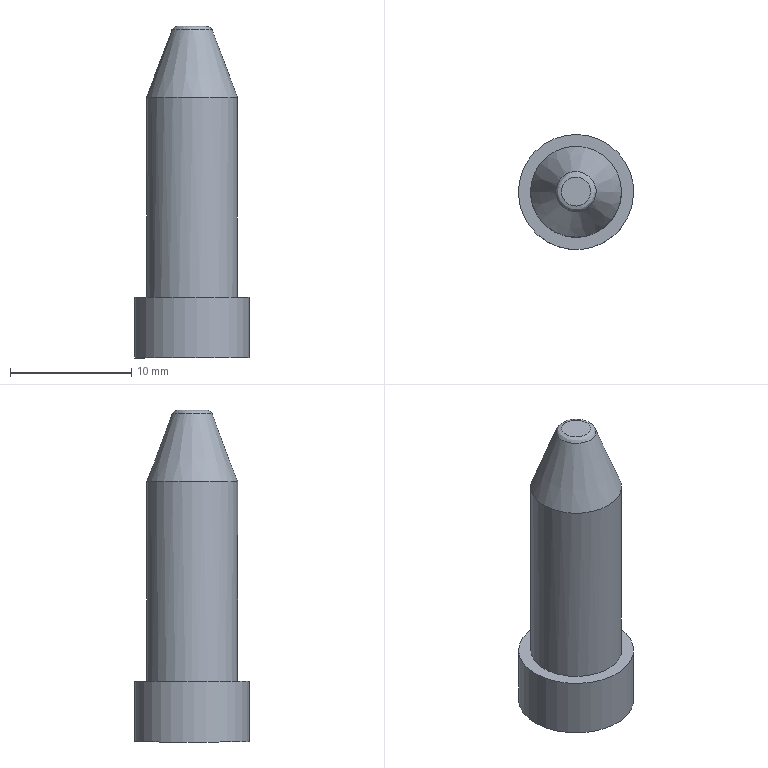Part | STEP file | gslz 2016.10.28-6_id1054_x_t | 1 solid | 7 faces | box 9.497 x 9.497 x 27.383 mm | volume 1219 mm3 | plane 3 | spline 2 | cylinder 1 | cone 1 | commonest cylinder face diameters 7.5 x1
STEP:
#1=CARTESIAN_POINT('',(19.769,170.458,47.));
#2=VERTEX_POINT('',#1);
#3=CARTESIAN_POINT('',(23.484,170.969,47.));
#4=DIRECTION('',(0.,0.,1.));
#5=DIRECTION('',(-0.9907,-0.1362,0.));
#6=AXIS2_PLACEMENT_3D('',#3,#4,#5);
#7=ELLIPSE('',#6,3.75,3.75);
#8=EDGE_CURVE('',#2,#2,#7,.T.);
#9=ORIENTED_EDGE('',*,*,#8,.T.);
#10=EDGE_LOOP('',(#9));
#11=FACE_BOUND('',#10,.T.);
#12=CARTESIAN_POINT('',(27.232,170.968,63.49));
#13=VERTEX_POINT('',#12);
#14=CARTESIAN_POINT('',(27.232,169.977,63.49));
#15=CARTESIAN_POINT('',(27.232,171.959,63.49));
#16=CARTESIAN_POINT('',(26.829,172.923,63.49));
#17=CARTESIAN_POINT('',(25.441,174.313,63.49));
#18=CARTESIAN_POINT('',(24.463,174.717,63.49));
#19=CARTESIAN_POINT('',(22.508,174.719,63.49));
#20=CARTESIAN_POINT('',(21.53,174.318,63.49));
#21=CARTESIAN_POINT('',(20.137,172.928,63.49));
#22=CARTESIAN_POINT('',(19.732,171.954,63.49));
#23=CARTESIAN_POINT('',(19.731,169.989,63.49));
#24=CARTESIAN_POINT('',(20.137,169.011,63.49));
#25=CARTESIAN_POINT('',(21.517,167.628,63.49));
#26=CARTESIAN_POINT('',(22.493,167.22,63.49));
#27=CARTESIAN_POINT('',(24.46,167.217,63.49));
#28=CARTESIAN_POINT('',(25.435,167.62,63.49));
#29=CARTESIAN_POINT('',(26.827,169.009,63.49));
#30=CARTESIAN_POINT('',(27.232,169.977,63.49));
#31=CARTESIAN_POINT('',(27.232,171.959,63.49));
#32=B_SPLINE_CURVE_WITH_KNOTS('',3,(#14,#15,#16,#17,#18,#19,#20,#21,#22,#23,#24,#25,#26,#27,#28,#29,#30,#31),.UNSPECIFIED.,.T.,.F.,(2,2,2,2,2,2,2,2,2,2,2),(-0.125,0.,0.125,0.25,0.375,0.5,0.625,0.75,0.875,1.,1.125),.UNSPECIFIED.);
#33=EDGE_CURVE('',#13,#13,#32,.T.);
#34=ORIENTED_EDGE('',*,*,#33,.F.);
#35=EDGE_LOOP('',(#34));
#36=FACE_BOUND('',#35,.T.);
#37=CARTESIAN_POINT('',(23.49,170.969,13.491));
#38=DIRECTION('',(-0.0001633,-0.00002245,1.));
#39=DIRECTION('',(1.,0.,0.0001633));
#40=AXIS2_PLACEMENT_3D('',#37,#38,#39);
#41=CYLINDRICAL_SURFACE('',#40,3.75);
#42=ADVANCED_FACE('',(#11,#36),#41,.T.);
#43=CARTESIAN_POINT('',(24.674,170.968,69.383));
#44=VERTEX_POINT('',#43);
#45=CARTESIAN_POINT('',(23.481,170.968,69.383));
#46=DIRECTION('',(0.0001633,-0.00002245,1.));
#47=DIRECTION('',(1.,-0.000000146,-0.0001633));
#48=AXIS2_PLACEMENT_3D('',#45,#46,#47);
#49=ELLIPSE('',#48,1.194,1.194);
#50=EDGE_CURVE('',#44,#44,#49,.T.);
#51=ORIENTED_EDGE('',*,*,#50,.T.);
#52=EDGE_LOOP('',(#51));
#53=FACE_OUTER_BOUND('',#52,.T.);
#54=CARTESIAN_POINT('',(-22.081,170.968,69.391));
#55=DIRECTION('',(0.0001633,-0.00002245,1.));
#56=DIRECTION('',(-1.,0.,0.0001633));
#57=AXIS2_PLACEMENT_3D('',#54,#55,#56);
#58=PLANE('',#57);
#59=ADVANCED_FACE('',(#53),#58,.T.);
#60=CARTESIAN_POINT('',(21.828,170.793,69.059));
#61=VERTEX_POINT('',#60);
#62=CARTESIAN_POINT('',(21.919,169.928,69.059));
#63=CARTESIAN_POINT('',(21.737,171.659,69.059));
#64=CARTESIAN_POINT('',(22.441,172.529,69.059));
#65=CARTESIAN_POINT('',(24.171,172.712,69.059));
#66=CARTESIAN_POINT('',(25.041,172.008,69.059));
#67=CARTESIAN_POINT('',(25.224,170.277,69.059));
#68=CARTESIAN_POINT('',(24.52,169.407,69.059));
#69=CARTESIAN_POINT('',(22.79,169.224,69.059));
#70=CARTESIAN_POINT('',(21.919,169.928,69.059));
#71=CARTESIAN_POINT('',(21.737,171.659,69.059));
#72=B_SPLINE_CURVE_WITH_KNOTS('',3,(#62,#63,#64,#65,#66,#67,#68,#69,#70,#71),.UNSPECIFIED.,.T.,.F.,(2,2,2,2,2,2,2),(-0.25,0.,0.25,0.5,0.75,1.,1.25),.UNSPECIFIED.);
#73=EDGE_CURVE('',#61,#61,#72,.T.);
#74=ORIENTED_EDGE('',*,*,#73,.T.);
#75=EDGE_LOOP('',(#74));
#76=FACE_BOUND('',#75,.T.);
#77=ORIENTED_EDGE('',*,*,#33,.T.);
#78=EDGE_LOOP('',(#77));
#79=FACE_BOUND('',#78,.T.);
#80=CARTESIAN_POINT('',(23.481,170.968,67.49));
#81=DIRECTION('',(0.0001633,0.00002245,-1.));
#82=DIRECTION('',(1.,-0.0000003,0.0001633));
#83=AXIS2_PLACEMENT_3D('',#80,#81,#82);
#84=CONICAL_SURFACE('',#83,2.25,20.556);
#85=ADVANCED_FACE('',(#76,#79),#84,.T.);
#86=CARTESIAN_POINT('',(18.873,169.831,47.));
#87=VERTEX_POINT('',#86);
#88=CARTESIAN_POINT('',(19.135,168.787,47.));
#89=CARTESIAN_POINT('',(18.833,169.993,47.));
#90=CARTESIAN_POINT('',(18.801,170.156,47.));
#91=CARTESIAN_POINT('',(18.609,171.554,47.));
#92=CARTESIAN_POINT('',(18.948,172.848,47.));
#93=CARTESIAN_POINT('',(20.451,174.829,47.));
#94=CARTESIAN_POINT('',(21.605,175.505,47.));
#95=CARTESIAN_POINT('',(24.069,175.844,47.));
#96=CARTESIAN_POINT('',(25.363,175.505,47.));
#97=CARTESIAN_POINT('',(27.345,174.002,47.));
#98=CARTESIAN_POINT('',(28.021,172.847,47.));
#99=CARTESIAN_POINT('',(28.359,170.383,47.));
#100=CARTESIAN_POINT('',(28.02,169.089,47.));
#101=CARTESIAN_POINT('',(26.518,167.108,47.));
#102=CARTESIAN_POINT('',(25.363,166.432,47.));
#103=CARTESIAN_POINT('',(22.899,166.093,47.));
#104=CARTESIAN_POINT('',(21.605,166.432,47.));
#105=CARTESIAN_POINT('',(19.756,167.834,47.));
#106=CARTESIAN_POINT('',(19.135,168.787,47.));
#107=CARTESIAN_POINT('',(18.833,169.993,47.));
#108=B_SPLINE_CURVE_WITH_KNOTS('',3,(#88,#89,#90,#91,#92,#93,#94,#95,#96,#97,#98,#99,#100,#101,#102,#103,#104,#105,#106,#107),.UNSPECIFIED.,.T.,.F.,(2,2,2,2,2,2,2,2,2,2,2,2),(-0.1082,0.,0.01676,0.1418,0.2668,0.3918,0.5168,0.6418,0.7668,0.8918,1.,1.017),.UNSPECIFIED.);
#109=EDGE_CURVE('',#87,#87,#108,.T.);
#110=ORIENTED_EDGE('',*,*,#109,.T.);
#111=EDGE_LOOP('',(#110));
#112=FACE_BOUND('',#111,.T.);
#113=CARTESIAN_POINT('',(18.873,169.831,42.));
#114=VERTEX_POINT('',#113);
#115=CARTESIAN_POINT('',(19.135,168.787,42.));
#116=CARTESIAN_POINT('',(18.833,169.993,42.));
#117=CARTESIAN_POINT('',(18.801,170.156,42.));
#118=CARTESIAN_POINT('',(18.609,171.554,42.));
#119=CARTESIAN_POINT('',(18.948,172.848,42.));
#120=CARTESIAN_POINT('',(20.451,174.829,42.));
#121=CARTESIAN_POINT('',(21.605,175.505,42.));
#122=CARTESIAN_POINT('',(24.069,175.844,42.));
#123=CARTESIAN_POINT('',(25.363,175.505,42.));
#124=CARTESIAN_POINT('',(27.345,174.002,42.));
#125=CARTESIAN_POINT('',(28.021,172.847,42.));
#126=CARTESIAN_POINT('',(28.359,170.383,42.));
#127=CARTESIAN_POINT('',(28.02,169.089,42.));
#128=CARTESIAN_POINT('',(26.518,167.108,42.));
#129=CARTESIAN_POINT('',(25.363,166.432,42.));
#130=CARTESIAN_POINT('',(22.899,166.093,42.));
#131=CARTESIAN_POINT('',(21.605,166.432,42.));
#132=CARTESIAN_POINT('',(19.756,167.834,42.));
#133=CARTESIAN_POINT('',(19.135,168.787,42.));
#134=CARTESIAN_POINT('',(18.833,169.993,42.));
#135=B_SPLINE_CURVE_WITH_KNOTS('',3,(#115,#116,#117,#118,#119,#120,#121,#122,#123,#124,#125,#126,#127,#128,#129,#130,#131,#132,#133,#134),.UNSPECIFIED.,.T.,.F.,(2,2,2,2,2,2,2,2,2,2,2,2),(-0.1082,0.,0.01676,0.1418,0.2668,0.3918,0.5168,0.6418,0.7668,0.8918,1.,1.017),.UNSPECIFIED.);
#136=EDGE_CURVE('',#114,#114,#135,.T.);
#137=ORIENTED_EDGE('',*,*,#136,.F.);
#138=EDGE_LOOP('',(#137));
#139=FACE_BOUND('',#138,.T.);
#140=CARTESIAN_POINT('',(18.948,169.09,47.));
#141=CARTESIAN_POINT('',(18.948,169.09,42.));
#142=CARTESIAN_POINT('',(18.609,171.554,47.));
#143=CARTESIAN_POINT('',(18.609,171.554,42.));
#144=CARTESIAN_POINT('',(18.948,172.848,47.));
#145=CARTESIAN_POINT('',(18.948,172.848,42.));
#146=CARTESIAN_POINT('',(20.451,174.829,47.));
#147=CARTESIAN_POINT('',(20.451,174.829,42.));
#148=CARTESIAN_POINT('',(21.605,175.505,47.));
#149=CARTESIAN_POINT('',(21.605,175.505,42.));
#150=CARTESIAN_POINT('',(24.069,175.844,47.));
#151=CARTESIAN_POINT('',(24.069,175.844,42.));
#152=CARTESIAN_POINT('',(25.363,175.505,47.));
#153=CARTESIAN_POINT('',(25.363,175.505,42.));
#154=CARTESIAN_POINT('',(27.345,174.002,47.));
#155=CARTESIAN_POINT('',(27.345,174.002,42.));
#156=CARTESIAN_POINT('',(28.021,172.847,47.));
#157=CARTESIAN_POINT('',(28.021,172.847,42.));
#158=CARTESIAN_POINT('',(28.359,170.383,47.));
#159=CARTESIAN_POINT('',(28.359,170.383,42.));
#160=CARTESIAN_POINT('',(28.02,169.089,47.));
#161=CARTESIAN_POINT('',(28.02,169.089,42.));
#162=CARTESIAN_POINT('',(26.518,167.108,47.));
#163=CARTESIAN_POINT('',(26.518,167.108,42.));
#164=CARTESIAN_POINT('',(25.363,166.432,47.));
#165=CARTESIAN_POINT('',(25.363,166.432,42.));
#166=CARTESIAN_POINT('',(22.899,166.093,47.));
#167=CARTESIAN_POINT('',(22.899,166.093,42.));
#168=CARTESIAN_POINT('',(21.605,166.432,47.));
#169=CARTESIAN_POINT('',(21.605,166.432,42.));
#170=CARTESIAN_POINT('',(19.623,167.935,47.));
#171=CARTESIAN_POINT('',(19.623,167.935,42.));
#172=CARTESIAN_POINT('',(18.948,169.09,47.));
#173=CARTESIAN_POINT('',(18.948,169.09,42.));
#174=CARTESIAN_POINT('',(18.609,171.554,47.));
#175=CARTESIAN_POINT('',(18.609,171.554,42.));
#176=B_SPLINE_SURFACE_WITH_KNOTS('',3,1,((#140,#141),(#142,#143),(#144,#145),(#146,#147),(#148,#149),(#150,#151),(#152,#153),(#154,#155),(#156,#157),(#158,#159),(#160,#161),(#162,#163),(#164,#165),(#166,#167),(#168,#169),(#170,#171),(#172,#173),(#174,#175)),.UNSPECIFIED.,.T.,.F.,.F.,(2,2,2,2,2,2,2,2,2,2,2),(2,2),(-0.125,0.,0.125,0.25,0.375,0.5,0.625,0.75,0.875,1.,1.125),(0.,1.),.UNSPECIFIED.);
#177=ADVANCED_FACE('',(#112,#139),#176,.T.);
#178=ORIENTED_EDGE('',*,*,#8,.F.);
#179=EDGE_LOOP('',(#178));
#180=FACE_BOUND('',#179,.T.);
#181=ORIENTED_EDGE('',*,*,#109,.F.);
#182=EDGE_LOOP('',(#181));
#183=FACE_BOUND('',#182,.T.);
#184=CARTESIAN_POINT('',(23.484,170.969,47.));
#185=DIRECTION('',(0.,0.,1.));
#186=DIRECTION('',(1.,-0.0000003,0.));
#187=AXIS2_PLACEMENT_3D('',#184,#185,#186);
#188=PLANE('',#187);
#189=ADVANCED_FACE('',(#180,#183),#188,.T.);
#190=ORIENTED_EDGE('',*,*,#136,.T.);
#191=EDGE_LOOP('',(#190));
#192=FACE_OUTER_BOUND('',#191,.T.);
#193=CARTESIAN_POINT('',(90.2,101.,42.));
#194=DIRECTION('',(0.,0.,1.));
#195=DIRECTION('',(1.,0.,0.));
#196=AXIS2_PLACEMENT_3D('',#193,#194,#195);
#197=PLANE('',#196);
#198=ADVANCED_FACE('',(#192),#197,.F.);
#199=ORIENTED_EDGE('',*,*,#50,.F.);
#200=EDGE_LOOP('',(#199));
#201=FACE_BOUND('',#200,.T.);
#202=ORIENTED_EDGE('',*,*,#73,.F.);
#203=EDGE_LOOP('',(#202));
#204=FACE_BOUND('',#203,.T.);
#205=CARTESIAN_POINT('',(25.142,170.533,69.059));
#206=CARTESIAN_POINT('',(25.021,170.565,69.383));
#207=CARTESIAN_POINT('',(24.674,170.656,69.383));
#208=CARTESIAN_POINT('',(25.142,171.403,69.059));
#209=CARTESIAN_POINT('',(25.021,171.371,69.383));
#210=CARTESIAN_POINT('',(24.674,171.28,69.383));
#211=CARTESIAN_POINT('',(24.963,171.835,69.059));
#212=CARTESIAN_POINT('',(24.855,171.772,69.383));
#213=CARTESIAN_POINT('',(24.546,171.591,69.383));
#214=CARTESIAN_POINT('',(24.348,172.451,69.059));
#215=CARTESIAN_POINT('',(24.285,172.342,69.383));
#216=CARTESIAN_POINT('',(24.104,172.033,69.383));
#217=CARTESIAN_POINT('',(23.916,172.63,69.059));
#218=CARTESIAN_POINT('',(23.884,172.508,69.383));
#219=CARTESIAN_POINT('',(23.793,172.162,69.383));
#220=CARTESIAN_POINT('',(23.046,172.63,69.059));
#221=CARTESIAN_POINT('',(23.077,172.508,69.383));
#222=CARTESIAN_POINT('',(23.168,172.162,69.383));
#223=CARTESIAN_POINT('',(22.613,172.451,69.059));
#224=CARTESIAN_POINT('',(22.677,172.342,69.383));
#225=CARTESIAN_POINT('',(22.858,172.033,69.383));
#226=CARTESIAN_POINT('',(21.998,171.835,69.059));
#227=CARTESIAN_POINT('',(22.107,171.772,69.383));
#228=CARTESIAN_POINT('',(22.416,171.591,69.383));
#229=CARTESIAN_POINT('',(21.819,171.403,69.059));
#230=CARTESIAN_POINT('',(21.941,171.371,69.383));
#231=CARTESIAN_POINT('',(22.287,171.28,69.383));
#232=CARTESIAN_POINT('',(21.819,170.533,69.059));
#233=CARTESIAN_POINT('',(21.941,170.565,69.383));
#234=CARTESIAN_POINT('',(22.287,170.656,69.383));
#235=CARTESIAN_POINT('',(21.998,170.101,69.059));
#236=CARTESIAN_POINT('',(22.107,170.164,69.383));
#237=CARTESIAN_POINT('',(22.416,170.345,69.383));
#238=CARTESIAN_POINT('',(22.613,169.485,69.059));
#239=CARTESIAN_POINT('',(22.677,169.594,69.383));
#240=CARTESIAN_POINT('',(22.858,169.903,69.383));
#241=CARTESIAN_POINT('',(23.046,169.306,69.059));
#242=CARTESIAN_POINT('',(23.077,169.428,69.383));
#243=CARTESIAN_POINT('',(23.168,169.774,69.383));
#244=CARTESIAN_POINT('',(23.916,169.306,69.059));
#245=CARTESIAN_POINT('',(23.884,169.428,69.383));
#246=CARTESIAN_POINT('',(23.793,169.774,69.383));
#247=CARTESIAN_POINT('',(24.348,169.485,69.059));
#248=CARTESIAN_POINT('',(24.285,169.594,69.383));
#249=CARTESIAN_POINT('',(24.104,169.903,69.383));
#250=CARTESIAN_POINT('',(24.963,170.101,69.059));
#251=CARTESIAN_POINT('',(24.855,170.164,69.383));
#252=CARTESIAN_POINT('',(24.546,170.345,69.383));
#253=CARTESIAN_POINT('',(25.142,170.533,69.059));
#254=CARTESIAN_POINT('',(25.021,170.565,69.383));
#255=CARTESIAN_POINT('',(24.674,170.656,69.383));
#256=CARTESIAN_POINT('',(25.142,171.403,69.059));
#257=CARTESIAN_POINT('',(25.021,171.371,69.383));
#258=CARTESIAN_POINT('',(24.674,171.28,69.383));
#259=(BOUNDED_SURFACE()B_SPLINE_SURFACE(3,2,((#205,#206,#207),(#208,#209,#210),(#211,#212,#213),(#214,#215,#216),(#217,#218,#219),(#220,#221,#222),(#223,#224,#225),(#226,#227,#228),(#229,#230,#231),(#232,#233,#234),(#235,#236,#237),(#238,#239,#240),(#241,#242,#243),(#244,#245,#246),(#247,#248,#249),(#250,#251,#252),(#253,#254,#255),(#256,#257,#258)),.UNSPECIFIED.,.T.,.F.,.F.)B_SPLINE_SURFACE_WITH_KNOTS((2,2,2,2,2,2,2,2,2,2,2),(3,3),(-0.125,0.,0.125,0.25,0.375,0.5,0.625,0.75,0.875,1.,1.125),(0.,1.),.UNSPECIFIED.)GEOMETRIC_REPRESENTATION_ITEM()RATIONAL_B_SPLINE_SURFACE(((1.,0.822,1.),(1.,0.822,1.),(1.,0.822,1.),(1.,0.822,1.),(1.,0.8219,1.),(1.,0.8219,1.),(1.,0.8219,1.),(1.,0.8218,1.),(1.,0.8218,1.),(1.,0.8218,1.),(1.,0.8218,1.),(1.,0.8219,1.),(1.,0.8219,1.),(1.,0.8219,1.),(1.,0.822,1.),(1.,0.822,1.),(1.,0.822,1.),(1.,0.822,1.)))REPRESENTATION_ITEM('')SURFACE());
#260=ADVANCED_FACE('',(#201,#204),#259,.T.);
#261=CLOSED_SHELL('',(#42,#59,#85,#177,#189,#198,#260));
#262=MANIFOLD_SOLID_BREP('',#261);
#263=(LENGTH_UNIT()NAMED_UNIT(*)SI_UNIT(.MILLI.,.METRE.));
#264=UNCERTAINTY_MEASURE_WITH_UNIT(LENGTH_MEASURE(0.071),#263,'','');
#265=(NAMED_UNIT(*)PLANE_ANGLE_UNIT()SI_UNIT($,.RADIAN.));
#266=PLANE_ANGLE_MEASURE_WITH_UNIT(PLANE_ANGLE_MEASURE(0.01745),#265);
#267=DIMENSIONAL_EXPONENTS(0.,0.,0.,0.,0.,0.,0.);
#268=(CONVERSION_BASED_UNIT('DEGREE',#266)NAMED_UNIT(#267)PLANE_ANGLE_UNIT());
#269=(NAMED_UNIT(*)SI_UNIT($,.STERADIAN.)SOLID_ANGLE_UNIT());
#270=(GEOMETRIC_REPRESENTATION_CONTEXT(3)GLOBAL_UNCERTAINTY_ASSIGNED_CONTEXT((#264))GLOBAL_UNIT_ASSIGNED_CONTEXT((#263,#268,#269))REPRESENTATION_CONTEXT('',''));
#271=ADVANCED_BREP_SHAPE_REPRESENTATION('',(#262),#270);